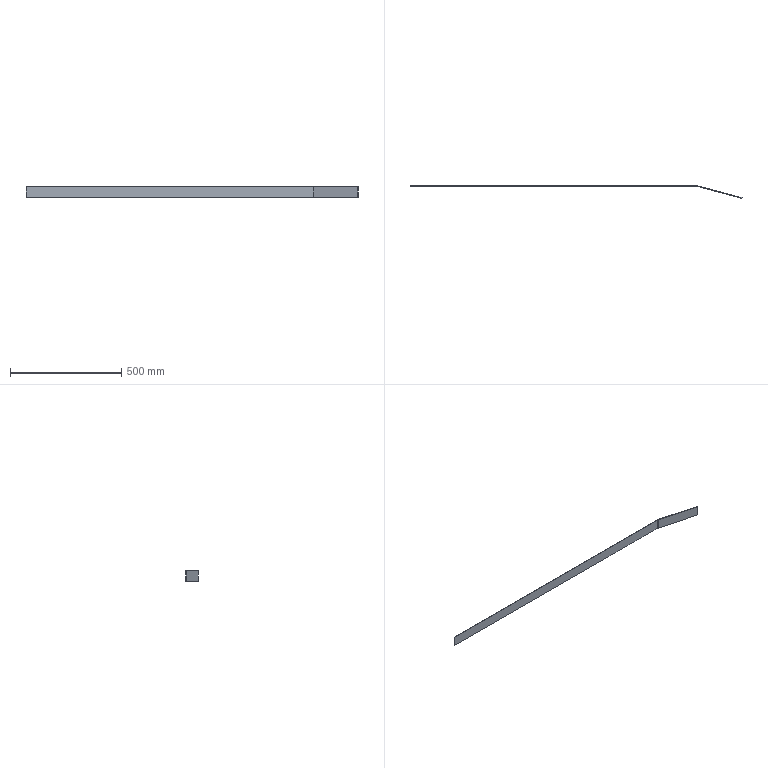Part | STEP file | SN10_017_001-01_CHAPA | 1 solid | 10 faces | box 1494 x 56.488 x 45 mm | volume 202588 mm3 | plane 8 | cylinder 2 | commonest cylinder face diameters 6 x1 12 x1
STEP:
#1=CARTESIAN_POINT('',(0.,0.,0.));
#2=DIRECTION('',(0.,0.,1.));
#3=DIRECTION('',(1.,0.,0.));
#4=AXIS2_PLACEMENT_3D('',#1,#2,#3);
#5=CARTESIAN_POINT('',(5024.,-1795.59,45.));
#6=VERTEX_POINT('',#5);
#7=CARTESIAN_POINT('',(5024.,-1795.59,90.));
#8=VERTEX_POINT('',#7);
#9=CARTESIAN_POINT('',(5024.,-1795.59,45.));
#10=DIRECTION('',(0.,0.,1.));
#11=VECTOR('',#10,1.);
#12=LINE('',#9,#11);
#13=CARTESIAN_POINT('',(5024.,-1795.59,45.));
#14=DIRECTION('',(0.2588,0.9659,0.));
#15=DIRECTION('',(0.,0.,1.));
#16=AXIS2_PLACEMENT_3D('',#13,#14,#15);
#17=PLANE('',#16);
#18=CARTESIAN_POINT('',(0.,0.));
#19=DIRECTION('',(1.,0.));
#20=VECTOR('',#19,1.);
#21=LINE('',#18,#20);
#22=(GEOMETRIC_REPRESENTATION_CONTEXT(2)PARAMETRIC_REPRESENTATION_CONTEXT()REPRESENTATION_CONTEXT('',''));
#23=DEFINITIONAL_REPRESENTATION('',(#21),#22);
#24=PCURVE('',#17,#23);
#25=CARTESIAN_POINT('',(5023.224,-1798.488,45.));
#26=DIRECTION('',(0.9659,-0.2588,0.));
#27=DIRECTION('',(0.,0.,-1.));
#28=AXIS2_PLACEMENT_3D('',#25,#26,#27);
#29=PLANE('',#28);
#30=CARTESIAN_POINT('',(0.,3.));
#31=DIRECTION('',(-1.,0.));
#32=VECTOR('',#31,1.);
#33=LINE('',#30,#32);
#34=(GEOMETRIC_REPRESENTATION_CONTEXT(2)PARAMETRIC_REPRESENTATION_CONTEXT()REPRESENTATION_CONTEXT('',''));
#35=DEFINITIONAL_REPRESENTATION('',(#33),#34);
#36=PCURVE('',#29,#35);
#37=SURFACE_CURVE('',#12,(#24,#36),.PCURVE_S1.);
#38=EDGE_CURVE('',#6,#8,#37,.T.);
#39=ORIENTED_EDGE('',*,*,#38,.F.);
#40=CARTESIAN_POINT('',(4824.763,-1742.204,45.));
#41=VERTEX_POINT('',#40);
#42=CARTESIAN_POINT('',(5024.,-1795.59,45.));
#43=DIRECTION('',(-0.9659,0.2588,0.));
#44=VECTOR('',#43,1.);
#45=LINE('',#42,#44);
#46=CARTESIAN_POINT('',(0.,0.000000004));
#47=DIRECTION('',(0.,-1.));
#48=VECTOR('',#47,1.);
#49=LINE('',#46,#48);
#50=(GEOMETRIC_REPRESENTATION_CONTEXT(2)PARAMETRIC_REPRESENTATION_CONTEXT()REPRESENTATION_CONTEXT('',''));
#51=DEFINITIONAL_REPRESENTATION('',(#49),#50);
#52=PCURVE('',#17,#51);
#53=CARTESIAN_POINT('',(0.,0.,45.));
#54=DIRECTION('',(0.,0.,1.));
#55=DIRECTION('',(1.,0.,0.));
#56=AXIS2_PLACEMENT_3D('',#53,#54,#55);
#57=PLANE('',#56);
#58=CARTESIAN_POINT('',(5024.,-1795.59));
#59=DIRECTION('',(-0.9659,0.2588));
#60=VECTOR('',#59,1.);
#61=LINE('',#58,#60);
#62=(GEOMETRIC_REPRESENTATION_CONTEXT(2)PARAMETRIC_REPRESENTATION_CONTEXT()REPRESENTATION_CONTEXT('',''));
#63=DEFINITIONAL_REPRESENTATION('',(#61),#62);
#64=PCURVE('',#57,#63);
#65=SURFACE_CURVE('',#45,(#52,#64),.PCURVE_S1.);
#66=EDGE_CURVE('',#6,#41,#65,.T.);
#67=ORIENTED_EDGE('',*,*,#66,.T.);
#68=CARTESIAN_POINT('',(4824.763,-1742.204,90.));
#69=VERTEX_POINT('',#68);
#70=CARTESIAN_POINT('',(4824.763,-1742.204,45.));
#71=DIRECTION('',(0.,0.,1.));
#72=VECTOR('',#71,1.);
#73=LINE('',#70,#72);
#74=CARTESIAN_POINT('',(0.,-206.265));
#75=DIRECTION('',(1.,0.));
#76=VECTOR('',#75,1.);
#77=LINE('',#74,#76);
#78=(GEOMETRIC_REPRESENTATION_CONTEXT(2)PARAMETRIC_REPRESENTATION_CONTEXT()REPRESENTATION_CONTEXT('',''));
#79=DEFINITIONAL_REPRESENTATION('',(#77),#78);
#80=PCURVE('',#17,#79);
#81=CARTESIAN_POINT('',(4823.21,-1748.,67.5));
#82=DIRECTION('',(0.,0.,1.));
#83=DIRECTION('',(0.2588,0.9659,0.));
#84=AXIS2_PLACEMENT_3D('',#81,#82,#83);
#85=CYLINDRICAL_SURFACE('',#84,6.);
#86=CARTESIAN_POINT('',(0.,-22.5));
#87=DIRECTION('',(0.,1.));
#88=VECTOR('',#87,1.);
#89=LINE('',#86,#88);
#90=(GEOMETRIC_REPRESENTATION_CONTEXT(2)PARAMETRIC_REPRESENTATION_CONTEXT()REPRESENTATION_CONTEXT('',''));
#91=DEFINITIONAL_REPRESENTATION('',(#89),#90);
#92=PCURVE('',#85,#91);
#93=SURFACE_CURVE('',#73,(#80,#92),.PCURVE_S1.);
#94=EDGE_CURVE('',#41,#69,#93,.T.);
#95=ORIENTED_EDGE('',*,*,#94,.T.);
#96=CARTESIAN_POINT('',(5024.,-1795.59,90.));
#97=DIRECTION('',(-0.9659,0.2588,0.));
#98=VECTOR('',#97,1.);
#99=LINE('',#96,#98);
#100=CARTESIAN_POINT('',(45.,0.000000004));
#101=DIRECTION('',(0.,-1.));
#102=VECTOR('',#101,1.);
#103=LINE('',#100,#102);
#104=(GEOMETRIC_REPRESENTATION_CONTEXT(2)PARAMETRIC_REPRESENTATION_CONTEXT()REPRESENTATION_CONTEXT('',''));
#105=DEFINITIONAL_REPRESENTATION('',(#103),#104);
#106=PCURVE('',#17,#105);
#107=CARTESIAN_POINT('',(0.,0.,90.));
#108=DIRECTION('',(0.,0.,1.));
#109=DIRECTION('',(1.,0.,0.));
#110=AXIS2_PLACEMENT_3D('',#107,#108,#109);
#111=PLANE('',#110);
#112=CARTESIAN_POINT('',(5024.,-1795.59));
#113=DIRECTION('',(-0.9659,0.2588));
#114=VECTOR('',#113,1.);
#115=LINE('',#112,#114);
#116=(GEOMETRIC_REPRESENTATION_CONTEXT(2)PARAMETRIC_REPRESENTATION_CONTEXT()REPRESENTATION_CONTEXT('',''));
#117=DEFINITIONAL_REPRESENTATION('',(#115),#116);
#118=PCURVE('',#111,#117);
#119=SURFACE_CURVE('',#99,(#106,#118),.PCURVE_S1.);
#120=EDGE_CURVE('',#8,#69,#119,.T.);
#121=ORIENTED_EDGE('',*,*,#120,.F.);
#122=EDGE_LOOP('',(#39,#67,#95,#121));
#123=FACE_BOUND('',#122,.T.);
#124=ADVANCED_FACE('',(#123),#17,.T.);
#125=ORIENTED_EDGE('',*,*,#94,.F.);
#126=CARTESIAN_POINT('',(4823.21,-1742.,45.));
#127=VERTEX_POINT('',#126);
#128=CARTESIAN_POINT('',(4823.21,-1748.,45.));
#129=DIRECTION('',(0.,0.,1.));
#130=DIRECTION('',(1.,0.,0.));
#131=AXIS2_PLACEMENT_3D('',#128,#129,#130);
#132=CIRCLE('',#131,6.);
#133=CARTESIAN_POINT('',(-1.309,-22.5));
#134=DIRECTION('',(1.,0.));
#135=VECTOR('',#134,1.);
#136=LINE('',#133,#135);
#137=(GEOMETRIC_REPRESENTATION_CONTEXT(2)PARAMETRIC_REPRESENTATION_CONTEXT()REPRESENTATION_CONTEXT('',''));
#138=DEFINITIONAL_REPRESENTATION('',(#136),#137);
#139=PCURVE('',#85,#138);
#140=CARTESIAN_POINT('',(4823.21,-1748.));
#141=DIRECTION('',(1.,0.));
#142=AXIS2_PLACEMENT_2D('',#140,#141);
#143=CIRCLE('',#142,6.);
#144=(GEOMETRIC_REPRESENTATION_CONTEXT(2)PARAMETRIC_REPRESENTATION_CONTEXT()REPRESENTATION_CONTEXT('',''));
#145=DEFINITIONAL_REPRESENTATION('',(#143),#144);
#146=PCURVE('',#57,#145);
#147=SURFACE_CURVE('',#132,(#139,#146),.PCURVE_S1.);
#148=EDGE_CURVE('',#41,#127,#147,.T.);
#149=ORIENTED_EDGE('',*,*,#148,.T.);
#150=CARTESIAN_POINT('',(4823.21,-1742.,90.));
#151=VERTEX_POINT('',#150);
#152=CARTESIAN_POINT('',(4823.21,-1742.,45.));
#153=DIRECTION('',(0.,0.,1.));
#154=VECTOR('',#153,1.);
#155=LINE('',#152,#154);
#156=CARTESIAN_POINT('',(0.2618,-22.5));
#157=DIRECTION('',(0.,1.));
#158=VECTOR('',#157,1.);
#159=LINE('',#156,#158);
#160=(GEOMETRIC_REPRESENTATION_CONTEXT(2)PARAMETRIC_REPRESENTATION_CONTEXT()REPRESENTATION_CONTEXT('',''));
#161=DEFINITIONAL_REPRESENTATION('',(#159),#160);
#162=PCURVE('',#85,#161);
#163=CARTESIAN_POINT('',(4823.21,-1742.,45.));
#164=DIRECTION('',(0.,1.,0.));
#165=DIRECTION('',(0.,0.,1.));
#166=AXIS2_PLACEMENT_3D('',#163,#164,#165);
#167=PLANE('',#166);
#168=CARTESIAN_POINT('',(0.,0.));
#169=DIRECTION('',(1.,0.));
#170=VECTOR('',#169,1.);
#171=LINE('',#168,#170);
#172=(GEOMETRIC_REPRESENTATION_CONTEXT(2)PARAMETRIC_REPRESENTATION_CONTEXT()REPRESENTATION_CONTEXT('',''));
#173=DEFINITIONAL_REPRESENTATION('',(#171),#172);
#174=PCURVE('',#167,#173);
#175=SURFACE_CURVE('',#155,(#162,#174),.PCURVE_S1.);
#176=EDGE_CURVE('',#127,#151,#175,.T.);
#177=ORIENTED_EDGE('',*,*,#176,.T.);
#178=CARTESIAN_POINT('',(4823.21,-1748.,90.));
#179=DIRECTION('',(0.,0.,1.));
#180=DIRECTION('',(1.,0.,0.));
#181=AXIS2_PLACEMENT_3D('',#178,#179,#180);
#182=CIRCLE('',#181,6.);
#183=CARTESIAN_POINT('',(-1.309,22.5));
#184=DIRECTION('',(1.,0.));
#185=VECTOR('',#184,1.);
#186=LINE('',#183,#185);
#187=(GEOMETRIC_REPRESENTATION_CONTEXT(2)PARAMETRIC_REPRESENTATION_CONTEXT()REPRESENTATION_CONTEXT('',''));
#188=DEFINITIONAL_REPRESENTATION('',(#186),#187);
#189=PCURVE('',#85,#188);
#190=CARTESIAN_POINT('',(4823.21,-1748.));
#191=DIRECTION('',(1.,0.));
#192=AXIS2_PLACEMENT_2D('',#190,#191);
#193=CIRCLE('',#192,6.);
#194=(GEOMETRIC_REPRESENTATION_CONTEXT(2)PARAMETRIC_REPRESENTATION_CONTEXT()REPRESENTATION_CONTEXT('',''));
#195=DEFINITIONAL_REPRESENTATION('',(#193),#194);
#196=PCURVE('',#111,#195);
#197=SURFACE_CURVE('',#182,(#189,#196),.PCURVE_S1.);
#198=EDGE_CURVE('',#69,#151,#197,.T.);
#199=ORIENTED_EDGE('',*,*,#198,.F.);
#200=EDGE_LOOP('',(#125,#149,#177,#199));
#201=FACE_BOUND('',#200,.T.);
#202=ADVANCED_FACE('',(#201),#85,.T.);
#203=ORIENTED_EDGE('',*,*,#176,.F.);
#204=CARTESIAN_POINT('',(3530.,-1742.,45.));
#205=VERTEX_POINT('',#204);
#206=CARTESIAN_POINT('',(4823.21,-1742.,45.));
#207=DIRECTION('',(-1.,0.,0.));
#208=VECTOR('',#207,1.);
#209=LINE('',#206,#208);
#210=CARTESIAN_POINT('',(0.,0.));
#211=DIRECTION('',(0.,-1.));
#212=VECTOR('',#211,1.);
#213=LINE('',#210,#212);
#214=(GEOMETRIC_REPRESENTATION_CONTEXT(2)PARAMETRIC_REPRESENTATION_CONTEXT()REPRESENTATION_CONTEXT('',''));
#215=DEFINITIONAL_REPRESENTATION('',(#213),#214);
#216=PCURVE('',#167,#215);
#217=CARTESIAN_POINT('',(4823.21,-1742.));
#218=DIRECTION('',(-1.,0.));
#219=VECTOR('',#218,1.);
#220=LINE('',#217,#219);
#221=(GEOMETRIC_REPRESENTATION_CONTEXT(2)PARAMETRIC_REPRESENTATION_CONTEXT()REPRESENTATION_CONTEXT('',''));
#222=DEFINITIONAL_REPRESENTATION('',(#220),#221);
#223=PCURVE('',#57,#222);
#224=SURFACE_CURVE('',#209,(#216,#223),.PCURVE_S1.);
#225=EDGE_CURVE('',#127,#205,#224,.T.);
#226=ORIENTED_EDGE('',*,*,#225,.T.);
#227=CARTESIAN_POINT('',(3530.,-1742.,90.));
#228=VERTEX_POINT('',#227);
#229=CARTESIAN_POINT('',(3530.,-1742.,45.));
#230=DIRECTION('',(0.,0.,1.));
#231=VECTOR('',#230,1.);
#232=LINE('',#229,#231);
#233=CARTESIAN_POINT('',(0.,-1293.21));
#234=DIRECTION('',(1.,0.));
#235=VECTOR('',#234,1.);
#236=LINE('',#233,#235);
#237=(GEOMETRIC_REPRESENTATION_CONTEXT(2)PARAMETRIC_REPRESENTATION_CONTEXT()REPRESENTATION_CONTEXT('',''));
#238=DEFINITIONAL_REPRESENTATION('',(#236),#237);
#239=PCURVE('',#167,#238);
#240=CARTESIAN_POINT('',(3530.,-1742.,45.));
#241=DIRECTION('',(-1.,0.,0.));
#242=DIRECTION('',(0.,0.,1.));
#243=AXIS2_PLACEMENT_3D('',#240,#241,#242);
#244=PLANE('',#243);
#245=CARTESIAN_POINT('',(0.,0.));
#246=DIRECTION('',(1.,0.));
#247=VECTOR('',#246,1.);
#248=LINE('',#245,#247);
#249=(GEOMETRIC_REPRESENTATION_CONTEXT(2)PARAMETRIC_REPRESENTATION_CONTEXT()REPRESENTATION_CONTEXT('',''));
#250=DEFINITIONAL_REPRESENTATION('',(#248),#249);
#251=PCURVE('',#244,#250);
#252=SURFACE_CURVE('',#232,(#239,#251),.PCURVE_S1.);
#253=EDGE_CURVE('',#205,#228,#252,.T.);
#254=ORIENTED_EDGE('',*,*,#253,.T.);
#255=CARTESIAN_POINT('',(4823.21,-1742.,90.));
#256=DIRECTION('',(-1.,0.,0.));
#257=VECTOR('',#256,1.);
#258=LINE('',#255,#257);
#259=CARTESIAN_POINT('',(45.,0.));
#260=DIRECTION('',(0.,-1.));
#261=VECTOR('',#260,1.);
#262=LINE('',#259,#261);
#263=(GEOMETRIC_REPRESENTATION_CONTEXT(2)PARAMETRIC_REPRESENTATION_CONTEXT()REPRESENTATION_CONTEXT('',''));
#264=DEFINITIONAL_REPRESENTATION('',(#262),#263);
#265=PCURVE('',#167,#264);
#266=CARTESIAN_POINT('',(4823.21,-1742.));
#267=DIRECTION('',(-1.,0.));
#268=VECTOR('',#267,1.);
#269=LINE('',#266,#268);
#270=(GEOMETRIC_REPRESENTATION_CONTEXT(2)PARAMETRIC_REPRESENTATION_CONTEXT()REPRESENTATION_CONTEXT('',''));
#271=DEFINITIONAL_REPRESENTATION('',(#269),#270);
#272=PCURVE('',#111,#271);
#273=SURFACE_CURVE('',#258,(#265,#272),.PCURVE_S1.);
#274=EDGE_CURVE('',#151,#228,#273,.T.);
#275=ORIENTED_EDGE('',*,*,#274,.F.);
#276=EDGE_LOOP('',(#203,#226,#254,#275));
#277=FACE_BOUND('',#276,.T.);
#278=ADVANCED_FACE('',(#277),#167,.T.);
#279=ORIENTED_EDGE('',*,*,#253,.F.);
#280=CARTESIAN_POINT('',(3530.,-1745.,45.));
#281=VERTEX_POINT('',#280);
#282=CARTESIAN_POINT('',(3530.,-1742.,45.));
#283=DIRECTION('',(0.,-1.,0.));
#284=VECTOR('',#283,1.);
#285=LINE('',#282,#284);
#286=CARTESIAN_POINT('',(0.,0.));
#287=DIRECTION('',(0.,-1.));
#288=VECTOR('',#287,1.);
#289=LINE('',#286,#288);
#290=(GEOMETRIC_REPRESENTATION_CONTEXT(2)PARAMETRIC_REPRESENTATION_CONTEXT()REPRESENTATION_CONTEXT('',''));
#291=DEFINITIONAL_REPRESENTATION('',(#289),#290);
#292=PCURVE('',#244,#291);
#293=CARTESIAN_POINT('',(3530.,-1742.));
#294=DIRECTION('',(0.,-1.));
#295=VECTOR('',#294,1.);
#296=LINE('',#293,#295);
#297=(GEOMETRIC_REPRESENTATION_CONTEXT(2)PARAMETRIC_REPRESENTATION_CONTEXT()REPRESENTATION_CONTEXT('',''));
#298=DEFINITIONAL_REPRESENTATION('',(#296),#297);
#299=PCURVE('',#57,#298);
#300=SURFACE_CURVE('',#285,(#292,#299),.PCURVE_S1.);
#301=EDGE_CURVE('',#205,#281,#300,.T.);
#302=ORIENTED_EDGE('',*,*,#301,.T.);
#303=CARTESIAN_POINT('',(3530.,-1745.,90.));
#304=VERTEX_POINT('',#303);
#305=CARTESIAN_POINT('',(3530.,-1745.,45.));
#306=DIRECTION('',(0.,0.,1.));
#307=VECTOR('',#306,1.);
#308=LINE('',#305,#307);
#309=CARTESIAN_POINT('',(0.,-3.));
#310=DIRECTION('',(1.,0.));
#311=VECTOR('',#310,1.);
#312=LINE('',#309,#311);
#313=(GEOMETRIC_REPRESENTATION_CONTEXT(2)PARAMETRIC_REPRESENTATION_CONTEXT()REPRESENTATION_CONTEXT('',''));
#314=DEFINITIONAL_REPRESENTATION('',(#312),#313);
#315=PCURVE('',#244,#314);
#316=CARTESIAN_POINT('',(4823.21,-1745.,45.));
#317=DIRECTION('',(0.,1.,0.));
#318=DIRECTION('',(0.,0.,1.));
#319=AXIS2_PLACEMENT_3D('',#316,#317,#318);
#320=PLANE('',#319);
#321=CARTESIAN_POINT('',(0.,-1293.21));
#322=DIRECTION('',(1.,0.));
#323=VECTOR('',#322,1.);
#324=LINE('',#321,#323);
#325=(GEOMETRIC_REPRESENTATION_CONTEXT(2)PARAMETRIC_REPRESENTATION_CONTEXT()REPRESENTATION_CONTEXT('',''));
#326=DEFINITIONAL_REPRESENTATION('',(#324),#325);
#327=PCURVE('',#320,#326);
#328=SURFACE_CURVE('',#308,(#315,#327),.PCURVE_S1.);
#329=EDGE_CURVE('',#281,#304,#328,.T.);
#330=ORIENTED_EDGE('',*,*,#329,.T.);
#331=CARTESIAN_POINT('',(3530.,-1742.,90.));
#332=DIRECTION('',(0.,-1.,0.));
#333=VECTOR('',#332,1.);
#334=LINE('',#331,#333);
#335=CARTESIAN_POINT('',(45.,0.));
#336=DIRECTION('',(0.,-1.));
#337=VECTOR('',#336,1.);
#338=LINE('',#335,#337);
#339=(GEOMETRIC_REPRESENTATION_CONTEXT(2)PARAMETRIC_REPRESENTATION_CONTEXT()REPRESENTATION_CONTEXT('',''));
#340=DEFINITIONAL_REPRESENTATION('',(#338),#339);
#341=PCURVE('',#244,#340);
#342=CARTESIAN_POINT('',(3530.,-1742.));
#343=DIRECTION('',(0.,-1.));
#344=VECTOR('',#343,1.);
#345=LINE('',#342,#344);
#346=(GEOMETRIC_REPRESENTATION_CONTEXT(2)PARAMETRIC_REPRESENTATION_CONTEXT()REPRESENTATION_CONTEXT('',''));
#347=DEFINITIONAL_REPRESENTATION('',(#345),#346);
#348=PCURVE('',#111,#347);
#349=SURFACE_CURVE('',#334,(#341,#348),.PCURVE_S1.);
#350=EDGE_CURVE('',#228,#304,#349,.T.);
#351=ORIENTED_EDGE('',*,*,#350,.F.);
#352=EDGE_LOOP('',(#279,#302,#330,#351));
#353=FACE_BOUND('',#352,.T.);
#354=ADVANCED_FACE('',(#353),#244,.T.);
#355=CARTESIAN_POINT('',(4823.21,-1745.,90.));
#356=VERTEX_POINT('',#355);
#357=CARTESIAN_POINT('',(4823.21,-1745.,90.));
#358=DIRECTION('',(-1.,0.,0.));
#359=VECTOR('',#358,1.);
#360=LINE('',#357,#359);
#361=CARTESIAN_POINT('',(45.,0.));
#362=DIRECTION('',(0.,-1.));
#363=VECTOR('',#362,1.);
#364=LINE('',#361,#363);
#365=(GEOMETRIC_REPRESENTATION_CONTEXT(2)PARAMETRIC_REPRESENTATION_CONTEXT()REPRESENTATION_CONTEXT('',''));
#366=DEFINITIONAL_REPRESENTATION('',(#364),#365);
#367=PCURVE('',#320,#366);
#368=CARTESIAN_POINT('',(4823.21,-1745.));
#369=DIRECTION('',(-1.,0.));
#370=VECTOR('',#369,1.);
#371=LINE('',#368,#370);
#372=(GEOMETRIC_REPRESENTATION_CONTEXT(2)PARAMETRIC_REPRESENTATION_CONTEXT()REPRESENTATION_CONTEXT('',''));
#373=DEFINITIONAL_REPRESENTATION('',(#371),#372);
#374=PCURVE('',#111,#373);
#375=SURFACE_CURVE('',#360,(#367,#374),.PCURVE_S1.);
#376=EDGE_CURVE('',#356,#304,#375,.T.);
#377=ORIENTED_EDGE('',*,*,#376,.T.);
#378=ORIENTED_EDGE('',*,*,#329,.F.);
#379=CARTESIAN_POINT('',(4823.21,-1745.,45.));
#380=VERTEX_POINT('',#379);
#381=CARTESIAN_POINT('',(4823.21,-1745.,45.));
#382=DIRECTION('',(-1.,0.,0.));
#383=VECTOR('',#382,1.);
#384=LINE('',#381,#383);
#385=CARTESIAN_POINT('',(0.,0.));
#386=DIRECTION('',(0.,-1.));
#387=VECTOR('',#386,1.);
#388=LINE('',#385,#387);
#389=(GEOMETRIC_REPRESENTATION_CONTEXT(2)PARAMETRIC_REPRESENTATION_CONTEXT()REPRESENTATION_CONTEXT('',''));
#390=DEFINITIONAL_REPRESENTATION('',(#388),#389);
#391=PCURVE('',#320,#390);
#392=CARTESIAN_POINT('',(4823.21,-1745.));
#393=DIRECTION('',(-1.,0.));
#394=VECTOR('',#393,1.);
#395=LINE('',#392,#394);
#396=(GEOMETRIC_REPRESENTATION_CONTEXT(2)PARAMETRIC_REPRESENTATION_CONTEXT()REPRESENTATION_CONTEXT('',''));
#397=DEFINITIONAL_REPRESENTATION('',(#395),#396);
#398=PCURVE('',#57,#397);
#399=SURFACE_CURVE('',#384,(#391,#398),.PCURVE_S1.);
#400=EDGE_CURVE('',#380,#281,#399,.T.);
#401=ORIENTED_EDGE('',*,*,#400,.F.);
#402=CARTESIAN_POINT('',(4823.21,-1745.,45.));
#403=DIRECTION('',(0.,0.,1.));
#404=VECTOR('',#403,1.);
#405=LINE('',#402,#404);
#406=CARTESIAN_POINT('',(0.,0.));
#407=DIRECTION('',(1.,0.));
#408=VECTOR('',#407,1.);
#409=LINE('',#406,#408);
#410=(GEOMETRIC_REPRESENTATION_CONTEXT(2)PARAMETRIC_REPRESENTATION_CONTEXT()REPRESENTATION_CONTEXT('',''));
#411=DEFINITIONAL_REPRESENTATION('',(#409),#410);
#412=PCURVE('',#320,#411);
#413=CARTESIAN_POINT('',(4823.21,-1748.,67.5));
#414=DIRECTION('',(0.,0.,1.));
#415=DIRECTION('',(0.2588,0.9659,0.));
#416=AXIS2_PLACEMENT_3D('',#413,#414,#415);
#417=CYLINDRICAL_SURFACE('',#416,3.);
#418=CARTESIAN_POINT('',(0.2618,-22.5));
#419=DIRECTION('',(0.,1.));
#420=VECTOR('',#419,1.);
#421=LINE('',#418,#420);
#422=(GEOMETRIC_REPRESENTATION_CONTEXT(2)PARAMETRIC_REPRESENTATION_CONTEXT()REPRESENTATION_CONTEXT('',''));
#423=DEFINITIONAL_REPRESENTATION('',(#421),#422);
#424=PCURVE('',#417,#423);
#425=SURFACE_CURVE('',#405,(#412,#424),.PCURVE_S1.);
#426=EDGE_CURVE('',#380,#356,#425,.T.);
#427=ORIENTED_EDGE('',*,*,#426,.T.);
#428=EDGE_LOOP('',(#377,#378,#401,#427));
#429=FACE_BOUND('',#428,.T.);
#430=ADVANCED_FACE('',(#429),#320,.F.);
#431=CARTESIAN_POINT('',(4823.987,-1745.102,45.));
#432=VERTEX_POINT('',#431);
#433=CARTESIAN_POINT('',(4823.987,-1745.102,90.));
#434=VERTEX_POINT('',#433);
#435=CARTESIAN_POINT('',(4823.987,-1745.102,45.));
#436=DIRECTION('',(0.,0.,1.));
#437=VECTOR('',#436,1.);
#438=LINE('',#435,#437);
#439=CARTESIAN_POINT('',(0.000000002,-22.5));
#440=DIRECTION('',(0.,1.));
#441=VECTOR('',#440,1.);
#442=LINE('',#439,#441);
#443=(GEOMETRIC_REPRESENTATION_CONTEXT(2)PARAMETRIC_REPRESENTATION_CONTEXT()REPRESENTATION_CONTEXT('',''));
#444=DEFINITIONAL_REPRESENTATION('',(#442),#443);
#445=PCURVE('',#417,#444);
#446=CARTESIAN_POINT('',(5023.224,-1798.488,45.));
#447=DIRECTION('',(0.2588,0.9659,0.));
#448=DIRECTION('',(0.,0.,1.));
#449=AXIS2_PLACEMENT_3D('',#446,#447,#448);
#450=PLANE('',#449);
#451=CARTESIAN_POINT('',(0.,-206.265));
#452=DIRECTION('',(1.,0.));
#453=VECTOR('',#452,1.);
#454=LINE('',#451,#453);
#455=(GEOMETRIC_REPRESENTATION_CONTEXT(2)PARAMETRIC_REPRESENTATION_CONTEXT()REPRESENTATION_CONTEXT('',''));
#456=DEFINITIONAL_REPRESENTATION('',(#454),#455);
#457=PCURVE('',#450,#456);
#458=SURFACE_CURVE('',#438,(#445,#457),.PCURVE_S1.);
#459=EDGE_CURVE('',#432,#434,#458,.T.);
#460=ORIENTED_EDGE('',*,*,#459,.F.);
#461=CARTESIAN_POINT('',(4823.21,-1748.,45.));
#462=DIRECTION('',(0.,0.,1.));
#463=DIRECTION('',(1.,0.,0.));
#464=AXIS2_PLACEMENT_3D('',#461,#462,#463);
#465=CIRCLE('',#464,3.);
#466=CARTESIAN_POINT('',(-1.309,-22.5));
#467=DIRECTION('',(1.,0.));
#468=VECTOR('',#467,1.);
#469=LINE('',#466,#468);
#470=(GEOMETRIC_REPRESENTATION_CONTEXT(2)PARAMETRIC_REPRESENTATION_CONTEXT()REPRESENTATION_CONTEXT('',''));
#471=DEFINITIONAL_REPRESENTATION('',(#469),#470);
#472=PCURVE('',#417,#471);
#473=CARTESIAN_POINT('',(4823.21,-1748.));
#474=DIRECTION('',(1.,0.));
#475=AXIS2_PLACEMENT_2D('',#473,#474);
#476=CIRCLE('',#475,3.);
#477=(GEOMETRIC_REPRESENTATION_CONTEXT(2)PARAMETRIC_REPRESENTATION_CONTEXT()REPRESENTATION_CONTEXT('',''));
#478=DEFINITIONAL_REPRESENTATION('',(#476),#477);
#479=PCURVE('',#57,#478);
#480=SURFACE_CURVE('',#465,(#472,#479),.PCURVE_S1.);
#481=EDGE_CURVE('',#432,#380,#480,.T.);
#482=ORIENTED_EDGE('',*,*,#481,.T.);
#483=ORIENTED_EDGE('',*,*,#426,.T.);
#484=CARTESIAN_POINT('',(4823.21,-1748.,90.));
#485=DIRECTION('',(0.,0.,1.));
#486=DIRECTION('',(1.,0.,0.));
#487=AXIS2_PLACEMENT_3D('',#484,#485,#486);
#488=CIRCLE('',#487,3.);
#489=CARTESIAN_POINT('',(-1.309,22.5));
#490=DIRECTION('',(1.,0.));
#491=VECTOR('',#490,1.);
#492=LINE('',#489,#491);
#493=(GEOMETRIC_REPRESENTATION_CONTEXT(2)PARAMETRIC_REPRESENTATION_CONTEXT()REPRESENTATION_CONTEXT('',''));
#494=DEFINITIONAL_REPRESENTATION('',(#492),#493);
#495=PCURVE('',#417,#494);
#496=CARTESIAN_POINT('',(4823.21,-1748.));
#497=DIRECTION('',(1.,0.));
#498=AXIS2_PLACEMENT_2D('',#496,#497);
#499=CIRCLE('',#498,3.);
#500=(GEOMETRIC_REPRESENTATION_CONTEXT(2)PARAMETRIC_REPRESENTATION_CONTEXT()REPRESENTATION_CONTEXT('',''));
#501=DEFINITIONAL_REPRESENTATION('',(#499),#500);
#502=PCURVE('',#111,#501);
#503=SURFACE_CURVE('',#488,(#495,#502),.PCURVE_S1.);
#504=EDGE_CURVE('',#434,#356,#503,.T.);
#505=ORIENTED_EDGE('',*,*,#504,.F.);
#506=EDGE_LOOP('',(#460,#482,#483,#505));
#507=FACE_BOUND('',#506,.F.);
#508=ADVANCED_FACE('',(#507),#417,.F.);
#509=CARTESIAN_POINT('',(5023.224,-1798.488,90.));
#510=VERTEX_POINT('',#509);
#511=CARTESIAN_POINT('',(5023.224,-1798.488,90.));
#512=DIRECTION('',(-0.9659,0.2588,0.));
#513=VECTOR('',#512,1.);
#514=LINE('',#511,#513);
#515=CARTESIAN_POINT('',(45.,0.000000001));
#516=DIRECTION('',(0.,-1.));
#517=VECTOR('',#516,1.);
#518=LINE('',#515,#517);
#519=(GEOMETRIC_REPRESENTATION_CONTEXT(2)PARAMETRIC_REPRESENTATION_CONTEXT()REPRESENTATION_CONTEXT('',''));
#520=DEFINITIONAL_REPRESENTATION('',(#518),#519);
#521=PCURVE('',#450,#520);
#522=CARTESIAN_POINT('',(5023.224,-1798.488));
#523=DIRECTION('',(-0.9659,0.2588));
#524=VECTOR('',#523,1.);
#525=LINE('',#522,#524);
#526=(GEOMETRIC_REPRESENTATION_CONTEXT(2)PARAMETRIC_REPRESENTATION_CONTEXT()REPRESENTATION_CONTEXT('',''));
#527=DEFINITIONAL_REPRESENTATION('',(#525),#526);
#528=PCURVE('',#111,#527);
#529=SURFACE_CURVE('',#514,(#521,#528),.PCURVE_S1.);
#530=EDGE_CURVE('',#510,#434,#529,.T.);
#531=ORIENTED_EDGE('',*,*,#530,.T.);
#532=ORIENTED_EDGE('',*,*,#459,.F.);
#533=CARTESIAN_POINT('',(5023.224,-1798.488,45.));
#534=VERTEX_POINT('',#533);
#535=CARTESIAN_POINT('',(5023.224,-1798.488,45.));
#536=DIRECTION('',(-0.9659,0.2588,0.));
#537=VECTOR('',#536,1.);
#538=LINE('',#535,#537);
#539=CARTESIAN_POINT('',(0.,0.000000001));
#540=DIRECTION('',(0.,-1.));
#541=VECTOR('',#540,1.);
#542=LINE('',#539,#541);
#543=(GEOMETRIC_REPRESENTATION_CONTEXT(2)PARAMETRIC_REPRESENTATION_CONTEXT()REPRESENTATION_CONTEXT('',''));
#544=DEFINITIONAL_REPRESENTATION('',(#542),#543);
#545=PCURVE('',#450,#544);
#546=CARTESIAN_POINT('',(5023.224,-1798.488));
#547=DIRECTION('',(-0.9659,0.2588));
#548=VECTOR('',#547,1.);
#549=LINE('',#546,#548);
#550=(GEOMETRIC_REPRESENTATION_CONTEXT(2)PARAMETRIC_REPRESENTATION_CONTEXT()REPRESENTATION_CONTEXT('',''));
#551=DEFINITIONAL_REPRESENTATION('',(#549),#550);
#552=PCURVE('',#57,#551);
#553=SURFACE_CURVE('',#538,(#545,#552),.PCURVE_S1.);
#554=EDGE_CURVE('',#534,#432,#553,.T.);
#555=ORIENTED_EDGE('',*,*,#554,.F.);
#556=CARTESIAN_POINT('',(5023.224,-1798.488,45.));
#557=DIRECTION('',(0.,0.,1.));
#558=VECTOR('',#557,1.);
#559=LINE('',#556,#558);
#560=CARTESIAN_POINT('',(0.,0.));
#561=DIRECTION('',(1.,0.));
#562=VECTOR('',#561,1.);
#563=LINE('',#560,#562);
#564=(GEOMETRIC_REPRESENTATION_CONTEXT(2)PARAMETRIC_REPRESENTATION_CONTEXT()REPRESENTATION_CONTEXT('',''));
#565=DEFINITIONAL_REPRESENTATION('',(#563),#564);
#566=PCURVE('',#450,#565);
#567=CARTESIAN_POINT('',(0.,0.));
#568=DIRECTION('',(-1.,0.));
#569=VECTOR('',#568,1.);
#570=LINE('',#567,#569);
#571=(GEOMETRIC_REPRESENTATION_CONTEXT(2)PARAMETRIC_REPRESENTATION_CONTEXT()REPRESENTATION_CONTEXT('',''));
#572=DEFINITIONAL_REPRESENTATION('',(#570),#571);
#573=PCURVE('',#29,#572);
#574=SURFACE_CURVE('',#559,(#566,#573),.PCURVE_S1.);
#575=EDGE_CURVE('',#534,#510,#574,.T.);
#576=ORIENTED_EDGE('',*,*,#575,.T.);
#577=EDGE_LOOP('',(#531,#532,#555,#576));
#578=FACE_BOUND('',#577,.T.);
#579=ADVANCED_FACE('',(#578),#450,.F.);
#580=ORIENTED_EDGE('',*,*,#575,.F.);
#581=CARTESIAN_POINT('',(5023.224,-1798.488,45.));
#582=DIRECTION('',(0.2588,0.9659,0.));
#583=VECTOR('',#582,1.);
#584=LINE('',#581,#583);
#585=CARTESIAN_POINT('',(0.,0.000000003));
#586=DIRECTION('',(0.,1.));
#587=VECTOR('',#586,1.);
#588=LINE('',#585,#587);
#589=(GEOMETRIC_REPRESENTATION_CONTEXT(2)PARAMETRIC_REPRESENTATION_CONTEXT()REPRESENTATION_CONTEXT('',''));
#590=DEFINITIONAL_REPRESENTATION('',(#588),#589);
#591=PCURVE('',#29,#590);
#592=CARTESIAN_POINT('',(5023.224,-1798.488));
#593=DIRECTION('',(0.2588,0.9659));
#594=VECTOR('',#593,1.);
#595=LINE('',#592,#594);
#596=(GEOMETRIC_REPRESENTATION_CONTEXT(2)PARAMETRIC_REPRESENTATION_CONTEXT()REPRESENTATION_CONTEXT('',''));
#597=DEFINITIONAL_REPRESENTATION('',(#595),#596);
#598=PCURVE('',#57,#597);
#599=SURFACE_CURVE('',#584,(#591,#598),.PCURVE_S1.);
#600=EDGE_CURVE('',#534,#6,#599,.T.);
#601=ORIENTED_EDGE('',*,*,#600,.T.);
#602=ORIENTED_EDGE('',*,*,#38,.T.);
#603=CARTESIAN_POINT('',(5023.224,-1798.488,90.));
#604=DIRECTION('',(0.2588,0.9659,0.));
#605=VECTOR('',#604,1.);
#606=LINE('',#603,#605);
#607=CARTESIAN_POINT('',(-45.,0.000000003));
#608=DIRECTION('',(0.,1.));
#609=VECTOR('',#608,1.);
#610=LINE('',#607,#609);
#611=(GEOMETRIC_REPRESENTATION_CONTEXT(2)PARAMETRIC_REPRESENTATION_CONTEXT()REPRESENTATION_CONTEXT('',''));
#612=DEFINITIONAL_REPRESENTATION('',(#610),#611);
#613=PCURVE('',#29,#612);
#614=CARTESIAN_POINT('',(5023.224,-1798.488));
#615=DIRECTION('',(0.2588,0.9659));
#616=VECTOR('',#615,1.);
#617=LINE('',#614,#616);
#618=(GEOMETRIC_REPRESENTATION_CONTEXT(2)PARAMETRIC_REPRESENTATION_CONTEXT()REPRESENTATION_CONTEXT('',''));
#619=DEFINITIONAL_REPRESENTATION('',(#617),#618);
#620=PCURVE('',#111,#619);
#621=SURFACE_CURVE('',#606,(#613,#620),.PCURVE_S1.);
#622=EDGE_CURVE('',#510,#8,#621,.T.);
#623=ORIENTED_EDGE('',*,*,#622,.F.);
#624=EDGE_LOOP('',(#580,#601,#602,#623));
#625=FACE_BOUND('',#624,.T.);
#626=ADVANCED_FACE('',(#625),#29,.T.);
#627=ORIENTED_EDGE('',*,*,#600,.F.);
#628=ORIENTED_EDGE('',*,*,#554,.T.);
#629=ORIENTED_EDGE('',*,*,#481,.T.);
#630=ORIENTED_EDGE('',*,*,#400,.T.);
#631=ORIENTED_EDGE('',*,*,#301,.F.);
#632=ORIENTED_EDGE('',*,*,#225,.F.);
#633=ORIENTED_EDGE('',*,*,#148,.F.);
#634=ORIENTED_EDGE('',*,*,#66,.F.);
#635=EDGE_LOOP('',(#627,#628,#629,#630,#631,#632,#633,#634));
#636=FACE_BOUND('',#635,.T.);
#637=ADVANCED_FACE('',(#636),#57,.F.);
#638=ORIENTED_EDGE('',*,*,#120,.T.);
#639=ORIENTED_EDGE('',*,*,#198,.T.);
#640=ORIENTED_EDGE('',*,*,#274,.T.);
#641=ORIENTED_EDGE('',*,*,#350,.T.);
#642=ORIENTED_EDGE('',*,*,#376,.F.);
#643=ORIENTED_EDGE('',*,*,#504,.F.);
#644=ORIENTED_EDGE('',*,*,#530,.F.);
#645=ORIENTED_EDGE('',*,*,#622,.T.);
#646=EDGE_LOOP('',(#638,#639,#640,#641,#642,#643,#644,#645));
#647=FACE_BOUND('',#646,.T.);
#648=ADVANCED_FACE('',(#647),#111,.T.);
#649=CLOSED_SHELL('',(#124,#202,#278,#354,#430,#508,#579,#626,#637,#648));
#650=MANIFOLD_SOLID_BREP('',#649);
#651=(LENGTH_UNIT()NAMED_UNIT(*)SI_UNIT(.MILLI.,.METRE.));
#652=UNCERTAINTY_MEASURE_WITH_UNIT(LENGTH_MEASURE(0.0000001),#651,'','');
#653=(NAMED_UNIT(*)PLANE_ANGLE_UNIT()SI_UNIT($,.RADIAN.));
#654=(NAMED_UNIT(*)SI_UNIT($,.STERADIAN.)SOLID_ANGLE_UNIT());
#655=(GEOMETRIC_REPRESENTATION_CONTEXT(3)GLOBAL_UNCERTAINTY_ASSIGNED_CONTEXT((#652))GLOBAL_UNIT_ASSIGNED_CONTEXT((#651,#653,#654))REPRESENTATION_CONTEXT('',''));
#656=ADVANCED_BREP_SHAPE_REPRESENTATION('',(#4,#650),#655);